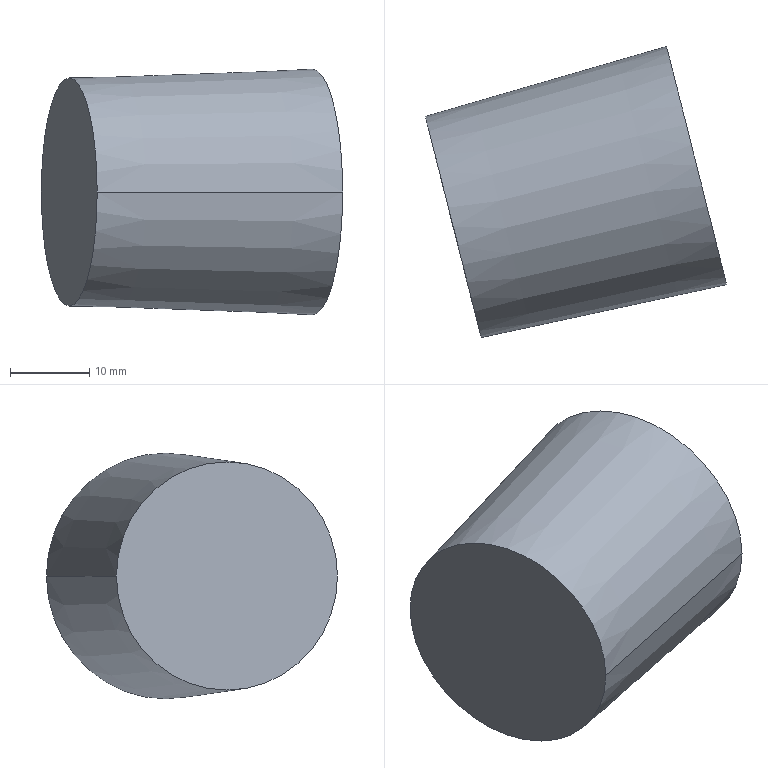Part | SolidWorks | features BaseBody 1 | 1 solid | 4 faces | box 37.94 x 36.648 x 30.927 mm | volume 22081 mm3 | plane 2 | cone 2
STEP:
#1=CARTESIAN_POINT('',(31.827,123.684,0.));
#2=VERTEX_POINT('',#1);
#3=CARTESIAN_POINT('',(39.396,93.697,0.));
#4=VERTEX_POINT('',#3);
#5=CARTESIAN_POINT('',(35.612,108.69,0.));
#6=DIRECTION('',(-0.9696,-0.2447,0.));
#7=DIRECTION('',(0.2447,-0.9696,0.));
#8=AXIS2_PLACEMENT_3D('',#5,#6,#7);
#9=CIRCLE('',#8,15.463);
#10=EDGE_CURVE('',#2,#4,#9,.T.);
#11=ORIENTED_EDGE('',*,*,#10,.F.);
#12=CARTESIAN_POINT('',(35.612,108.69,0.));
#13=DIRECTION('',(-0.9696,-0.2447,0.));
#14=DIRECTION('',(0.2447,-0.9696,0.));
#15=AXIS2_PLACEMENT_3D('',#12,#13,#14);
#16=CIRCLE('',#15,15.463);
#17=EDGE_CURVE('',#4,#2,#16,.T.);
#18=ORIENTED_EDGE('',*,*,#17,.F.);
#19=EDGE_LOOP('',(#11,#18));
#20=FACE_OUTER_BOUND('',#19,.T.);
#21=CARTESIAN_POINT('',(35.612,108.69,0.));
#22=DIRECTION('',(-0.9696,-0.2447,0.));
#23=DIRECTION('',(0.2447,-0.9696,0.));
#24=AXIS2_PLACEMENT_3D('',#21,#22,#23);
#25=PLANE('',#24);
#26=ADVANCED_FACE('',(#20),#25,.F.);
#27=CARTESIAN_POINT('',(8.484,87.036,0.));
#28=VERTEX_POINT('',#27);
#29=CARTESIAN_POINT('',(8.484,87.036,0.));
#30=DIRECTION('',(0.9776,0.2107,0.));
#31=VECTOR('',#30,1000.);
#32=LINE('',#29,#31);
#33=EDGE_CURVE('',#28,#4,#32,.T.);
#34=ORIENTED_EDGE('',*,*,#33,.T.);
#35=ORIENTED_EDGE('',*,*,#17,.T.);
#36=CARTESIAN_POINT('',(1.456,114.876,0.));
#37=VERTEX_POINT('',#36);
#38=CARTESIAN_POINT('',(1.456,114.876,0.));
#39=DIRECTION('',(0.9604,0.2785,0.));
#40=VECTOR('',#39,1000.);
#41=LINE('',#38,#40);
#42=EDGE_CURVE('',#37,#2,#41,.T.);
#43=ORIENTED_EDGE('',*,*,#42,.F.);
#44=CARTESIAN_POINT('',(4.97,100.956,0.));
#45=DIRECTION('',(-0.9696,-0.2447,0.));
#46=DIRECTION('',(0.2447,-0.9696,0.));
#47=AXIS2_PLACEMENT_3D('',#44,#45,#46);
#48=CIRCLE('',#47,14.357);
#49=EDGE_CURVE('',#28,#37,#48,.T.);
#50=ORIENTED_EDGE('',*,*,#49,.F.);
#51=EDGE_LOOP('',(#34,#35,#43,#50));
#52=FACE_OUTER_BOUND('',#51,.T.);
#53=CARTESIAN_POINT('',(35.612,108.69,0.));
#54=DIRECTION('',(0.9696,0.2447,0.));
#55=DIRECTION('',(0.,0.,-1.));
#56=AXIS2_PLACEMENT_3D('',#53,#54,#55);
#57=CONICAL_SURFACE('',#56,15.463,0.03501);
#58=ADVANCED_FACE('',(#52),#57,.T.);
#59=ORIENTED_EDGE('',*,*,#49,.T.);
#60=CARTESIAN_POINT('',(4.97,100.956,0.));
#61=DIRECTION('',(-0.9696,-0.2447,0.));
#62=DIRECTION('',(0.2447,-0.9696,0.));
#63=AXIS2_PLACEMENT_3D('',#60,#61,#62);
#64=CIRCLE('',#63,14.357);
#65=EDGE_CURVE('',#37,#28,#64,.T.);
#66=ORIENTED_EDGE('',*,*,#65,.T.);
#67=EDGE_LOOP('',(#59,#66));
#68=FACE_OUTER_BOUND('',#67,.T.);
#69=CARTESIAN_POINT('',(8.484,87.036,0.));
#70=DIRECTION('',(0.9696,0.2447,0.));
#71=DIRECTION('',(-0.2447,0.9696,0.));
#72=AXIS2_PLACEMENT_3D('',#69,#70,#71);
#73=PLANE('',#72);
#74=ADVANCED_FACE('',(#68),#73,.F.);
#75=ORIENTED_EDGE('',*,*,#33,.F.);
#76=ORIENTED_EDGE('',*,*,#65,.F.);
#77=ORIENTED_EDGE('',*,*,#42,.T.);
#78=ORIENTED_EDGE('',*,*,#10,.T.);
#79=EDGE_LOOP('',(#75,#76,#77,#78));
#80=FACE_OUTER_BOUND('',#79,.T.);
#81=CARTESIAN_POINT('',(35.612,108.69,0.));
#82=DIRECTION('',(0.9696,0.2447,0.));
#83=DIRECTION('',(0.,0.,1.));
#84=AXIS2_PLACEMENT_3D('',#81,#82,#83);
#85=CONICAL_SURFACE('',#84,15.463,0.03501);
#86=ADVANCED_FACE('',(#80),#85,.T.);
#87=CLOSED_SHELL('',(#26,#58,#74,#86));
#88=MANIFOLD_SOLID_BREP('',#87);
#89=CARTESIAN_POINT('',(0.,0.,0.));
#90=DIRECTION('',(0.,0.,1.));
#91=DIRECTION('',(1.,0.,0.));
#92=AXIS2_PLACEMENT_3D('',#89,#90,#91);
#93=(LENGTH_UNIT()NAMED_UNIT(*)SI_UNIT(.MILLI.,.METRE.));
#94=UNCERTAINTY_MEASURE_WITH_UNIT(LENGTH_MEASURE(0.00001),#93,'','');
#95=(NAMED_UNIT(*)PLANE_ANGLE_UNIT()SI_UNIT($,.RADIAN.));
#96=(NAMED_UNIT(*)SI_UNIT($,.STERADIAN.)SOLID_ANGLE_UNIT());
#97=(GEOMETRIC_REPRESENTATION_CONTEXT(3)GLOBAL_UNCERTAINTY_ASSIGNED_CONTEXT((#94))GLOBAL_UNIT_ASSIGNED_CONTEXT((#93,#95,#96))REPRESENTATION_CONTEXT('',''));
#98=ADVANCED_BREP_SHAPE_REPRESENTATION('',(#88,#92),#97);